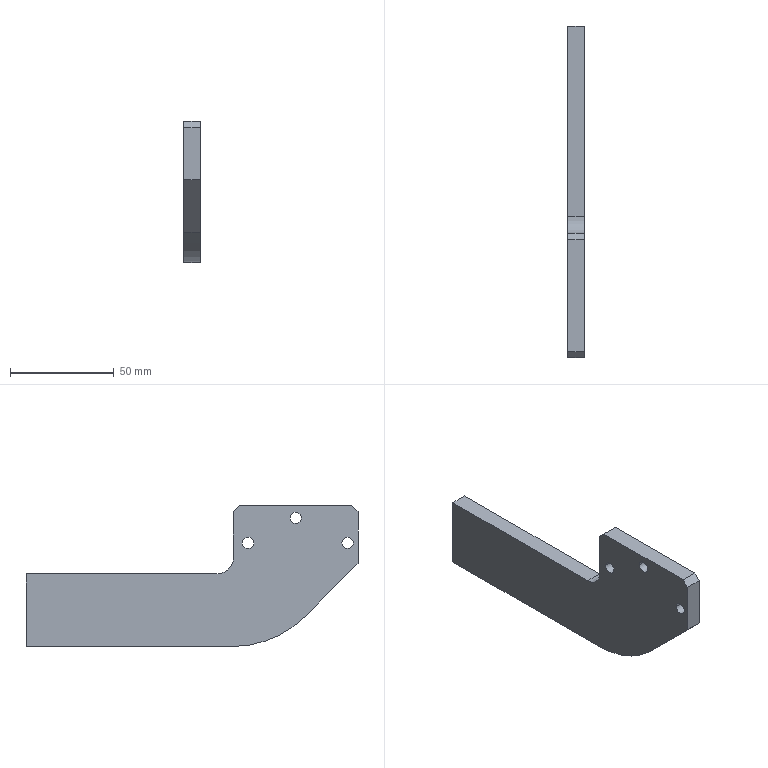Part | STEP file | support plate 11 | 1 solid | 27 faces | box 8 x 160 x 68 mm | volume 53075 mm3 | cylinder 12 | plane 11 | cone 4 | commonest cylinder face diameters 5.5 x6 3.3 x4 16 x1 100 x1